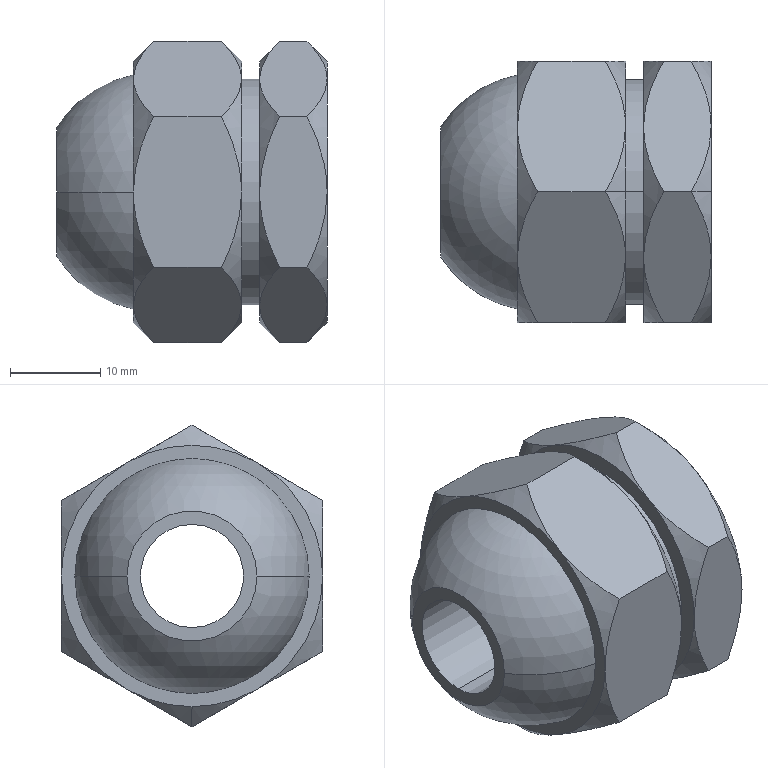Part | SolidWorks | features ICE 4, RevCut 1, Revolution 1 | 1 solid | 51 faces | box 30 x 29 x 33.486 mm | volume 15189 mm3 | cone 28 | plane 17 | cylinder 4 | sphere 2 | commonest cylinder face diameters 11.445 x2 25 x2